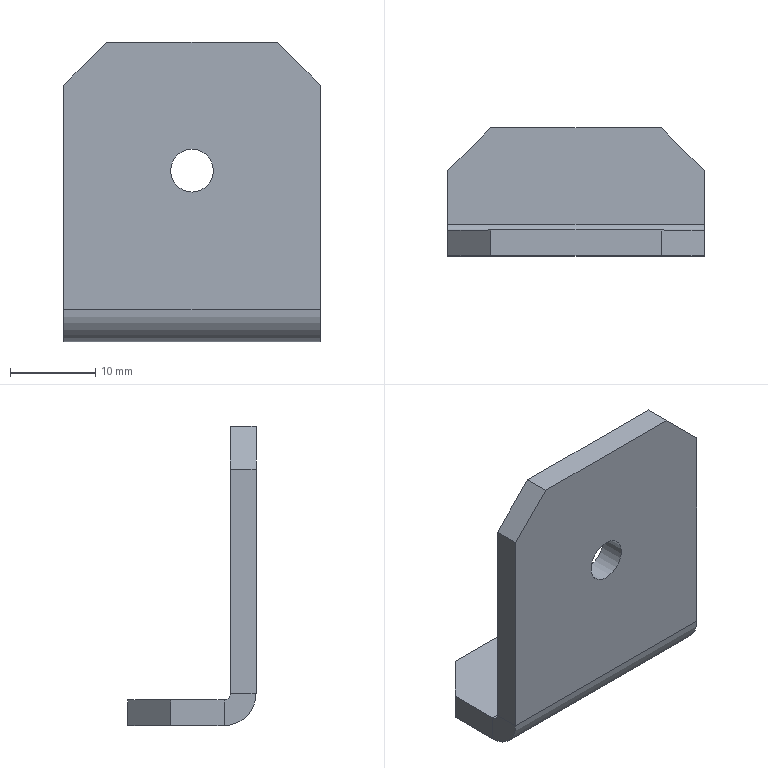Part | NX | 1 solid | 19 faces | box 30 x 15 x 35 mm | volume 3934 mm3 | plane 16 | cylinder 3 | commonest cylinder face diameters 1.5 x1 5 x1 7.5 x1
STEP:
#1=CARTESIAN_POINT('',(15.,0.,3.75));
#2=VERTEX_POINT('',#1);
#3=CARTESIAN_POINT('',(15.,3.,3.75));
#4=VERTEX_POINT('',#3);
#5=CARTESIAN_POINT('',(15.,0.,3.75));
#6=DIRECTION('',(0.,1.,0.));
#7=VECTOR('',#6,1000.);
#8=LINE('',#5,#7);
#9=EDGE_CURVE('',#2,#4,#8,.T.);
#10=ORIENTED_EDGE('',*,*,#9,.F.);
#11=CARTESIAN_POINT('',(15.,3.75,0.));
#12=VERTEX_POINT('',#11);
#13=CARTESIAN_POINT('',(15.,3.75,3.75));
#14=DIRECTION('',(1.,0.,0.));
#15=DIRECTION('',(0.,0.,-1.));
#16=AXIS2_PLACEMENT_3D('',#13,#14,#15);
#17=CIRCLE('',#16,3.75);
#18=EDGE_CURVE('',#12,#2,#17,.F.);
#19=ORIENTED_EDGE('',*,*,#18,.F.);
#20=CARTESIAN_POINT('',(15.,3.75,3.));
#21=VERTEX_POINT('',#20);
#22=CARTESIAN_POINT('',(15.,3.75,3.));
#23=DIRECTION('',(0.,0.,-1.));
#24=VECTOR('',#23,1000.);
#25=LINE('',#22,#24);
#26=EDGE_CURVE('',#21,#12,#25,.T.);
#27=ORIENTED_EDGE('',*,*,#26,.F.);
#28=CARTESIAN_POINT('',(15.,3.75,3.75));
#29=DIRECTION('',(1.,0.,0.));
#30=DIRECTION('',(0.,0.,-1.));
#31=AXIS2_PLACEMENT_3D('',#28,#29,#30);
#32=CIRCLE('',#31,0.75);
#33=EDGE_CURVE('',#21,#4,#32,.F.);
#34=ORIENTED_EDGE('',*,*,#33,.T.);
#35=EDGE_LOOP('',(#10,#19,#27,#34));
#36=FACE_BOUND('',#35,.T.);
#37=CARTESIAN_POINT('',(15.,0.,3.75));
#38=DIRECTION('',(1.,0.,0.));
#39=DIRECTION('',(0.,0.,-1.));
#40=AXIS2_PLACEMENT_3D('',#37,#38,#39);
#41=PLANE('',#40);
#42=ADVANCED_FACE('',(#36),#41,.T.);
#43=CARTESIAN_POINT('',(15.,3.,30.));
#44=VERTEX_POINT('',#43);
#45=CARTESIAN_POINT('',(15.,3.,0.));
#46=DIRECTION('',(0.,0.,1.));
#47=VECTOR('',#46,1000.);
#48=LINE('',#45,#47);
#49=EDGE_CURVE('',#4,#44,#48,.T.);
#50=ORIENTED_EDGE('',*,*,#49,.T.);
#51=CARTESIAN_POINT('',(15.,0.,30.));
#52=VERTEX_POINT('',#51);
#53=CARTESIAN_POINT('',(15.,3.75,30.));
#54=DIRECTION('',(0.,-1.,0.));
#55=VECTOR('',#54,1000.);
#56=LINE('',#53,#55);
#57=EDGE_CURVE('',#44,#52,#56,.T.);
#58=ORIENTED_EDGE('',*,*,#57,.T.);
#59=CARTESIAN_POINT('',(15.,0.,0.));
#60=DIRECTION('',(0.,0.,1.));
#61=VECTOR('',#60,1000.);
#62=LINE('',#59,#61);
#63=EDGE_CURVE('',#2,#52,#62,.T.);
#64=ORIENTED_EDGE('',*,*,#63,.F.);
#65=ORIENTED_EDGE('',*,*,#9,.T.);
#66=EDGE_LOOP('',(#50,#58,#64,#65));
#67=FACE_BOUND('',#66,.T.);
#68=CARTESIAN_POINT('',(15.,3.75,3.));
#69=DIRECTION('',(1.,0.,0.));
#70=DIRECTION('',(0.,0.,-1.));
#71=AXIS2_PLACEMENT_3D('',#68,#69,#70);
#72=PLANE('',#71);
#73=ADVANCED_FACE('',(#67),#72,.T.);
#74=CARTESIAN_POINT('',(-15.,3.75,0.));
#75=VERTEX_POINT('',#74);
#76=CARTESIAN_POINT('',(-15.,3.75,3.));
#77=VERTEX_POINT('',#76);
#78=CARTESIAN_POINT('',(-15.,3.75,0.));
#79=DIRECTION('',(0.,0.,1.));
#80=VECTOR('',#79,1000.);
#81=LINE('',#78,#80);
#82=EDGE_CURVE('',#75,#77,#81,.T.);
#83=ORIENTED_EDGE('',*,*,#82,.F.);
#84=CARTESIAN_POINT('',(-15.,0.,3.75));
#85=VERTEX_POINT('',#84);
#86=CARTESIAN_POINT('',(-15.,3.75,3.75));
#87=DIRECTION('',(1.,0.,0.));
#88=DIRECTION('',(0.,0.,-1.));
#89=AXIS2_PLACEMENT_3D('',#86,#87,#88);
#90=CIRCLE('',#89,3.75);
#91=EDGE_CURVE('',#75,#85,#90,.F.);
#92=ORIENTED_EDGE('',*,*,#91,.T.);
#93=CARTESIAN_POINT('',(-15.,3.,3.75));
#94=VERTEX_POINT('',#93);
#95=CARTESIAN_POINT('',(-15.,3.,3.75));
#96=DIRECTION('',(0.,-1.,0.));
#97=VECTOR('',#96,1000.);
#98=LINE('',#95,#97);
#99=EDGE_CURVE('',#94,#85,#98,.T.);
#100=ORIENTED_EDGE('',*,*,#99,.F.);
#101=CARTESIAN_POINT('',(-15.,3.75,3.75));
#102=DIRECTION('',(1.,0.,0.));
#103=DIRECTION('',(0.,0.,-1.));
#104=AXIS2_PLACEMENT_3D('',#101,#102,#103);
#105=CIRCLE('',#104,0.75);
#106=EDGE_CURVE('',#77,#94,#105,.F.);
#107=ORIENTED_EDGE('',*,*,#106,.F.);
#108=EDGE_LOOP('',(#83,#92,#100,#107));
#109=FACE_BOUND('',#108,.T.);
#110=CARTESIAN_POINT('',(-15.,3.75,0.));
#111=DIRECTION('',(-1.,0.,0.));
#112=DIRECTION('',(0.,0.,1.));
#113=AXIS2_PLACEMENT_3D('',#110,#111,#112);
#114=PLANE('',#113);
#115=ADVANCED_FACE('',(#109),#114,.T.);
#116=CARTESIAN_POINT('',(-15.,10.,3.));
#117=VERTEX_POINT('',#116);
#118=CARTESIAN_POINT('',(-15.,15.,3.));
#119=DIRECTION('',(0.,-1.,0.));
#120=VECTOR('',#119,1000.);
#121=LINE('',#118,#120);
#122=EDGE_CURVE('',#117,#77,#121,.T.);
#123=ORIENTED_EDGE('',*,*,#122,.F.);
#124=CARTESIAN_POINT('',(-15.,10.,0.));
#125=VERTEX_POINT('',#124);
#126=CARTESIAN_POINT('',(-15.,10.,3.75));
#127=DIRECTION('',(0.,0.,-1.));
#128=VECTOR('',#127,1000.);
#129=LINE('',#126,#128);
#130=EDGE_CURVE('',#117,#125,#129,.T.);
#131=ORIENTED_EDGE('',*,*,#130,.T.);
#132=CARTESIAN_POINT('',(-15.,15.,0.));
#133=DIRECTION('',(0.,-1.,0.));
#134=VECTOR('',#133,1000.);
#135=LINE('',#132,#134);
#136=EDGE_CURVE('',#125,#75,#135,.T.);
#137=ORIENTED_EDGE('',*,*,#136,.T.);
#138=ORIENTED_EDGE('',*,*,#82,.T.);
#139=EDGE_LOOP('',(#123,#131,#137,#138));
#140=FACE_BOUND('',#139,.T.);
#141=CARTESIAN_POINT('',(-15.,3.,3.75));
#142=DIRECTION('',(-1.,0.,0.));
#143=DIRECTION('',(0.,0.,1.));
#144=AXIS2_PLACEMENT_3D('',#141,#142,#143);
#145=PLANE('',#144);
#146=ADVANCED_FACE('',(#140),#145,.T.);
#147=CARTESIAN_POINT('',(0.,3.,17.5));
#148=VERTEX_POINT('',#147);
#149=CARTESIAN_POINT('',(0.,3.,20.));
#150=DIRECTION('',(0.,-1.,0.));
#151=DIRECTION('',(0.,0.,-1.));
#152=AXIS2_PLACEMENT_3D('',#149,#150,#151);
#153=CIRCLE('',#152,2.5);
#154=EDGE_CURVE('',#148,#148,#153,.T.);
#155=ORIENTED_EDGE('',*,*,#154,.T.);
#156=EDGE_LOOP('',(#155));
#157=FACE_BOUND('',#156,.T.);
#158=CARTESIAN_POINT('',(10.,3.,35.));
#159=VERTEX_POINT('',#158);
#160=CARTESIAN_POINT('',(-10.,3.,35.));
#161=VERTEX_POINT('',#160);
#162=CARTESIAN_POINT('',(15.,3.,35.));
#163=DIRECTION('',(-1.,0.,0.));
#164=VECTOR('',#163,1000.);
#165=LINE('',#162,#164);
#166=EDGE_CURVE('',#159,#161,#165,.T.);
#167=ORIENTED_EDGE('',*,*,#166,.F.);
#168=CARTESIAN_POINT('',(10.,3.,35.));
#169=DIRECTION('',(-0.7071,0.,0.7071));
#170=VECTOR('',#169,1000.);
#171=LINE('',#168,#170);
#172=EDGE_CURVE('',#159,#44,#171,.F.);
#173=ORIENTED_EDGE('',*,*,#172,.T.);
#174=ORIENTED_EDGE('',*,*,#49,.F.);
#175=CARTESIAN_POINT('',(15.,3.,3.75));
#176=DIRECTION('',(-1.,0.,0.));
#177=VECTOR('',#176,1000.);
#178=LINE('',#175,#177);
#179=EDGE_CURVE('',#4,#94,#178,.T.);
#180=ORIENTED_EDGE('',*,*,#179,.T.);
#181=CARTESIAN_POINT('',(-15.,3.,30.));
#182=VERTEX_POINT('',#181);
#183=CARTESIAN_POINT('',(-15.,3.,0.));
#184=DIRECTION('',(0.,0.,1.));
#185=VECTOR('',#184,1000.);
#186=LINE('',#183,#185);
#187=EDGE_CURVE('',#94,#182,#186,.T.);
#188=ORIENTED_EDGE('',*,*,#187,.T.);
#189=CARTESIAN_POINT('',(-15.,3.,30.));
#190=DIRECTION('',(0.7071,0.,0.7071));
#191=VECTOR('',#190,1000.);
#192=LINE('',#189,#191);
#193=EDGE_CURVE('',#182,#161,#192,.T.);
#194=ORIENTED_EDGE('',*,*,#193,.T.);
#195=EDGE_LOOP('',(#167,#173,#174,#180,#188,#194));
#196=FACE_BOUND('',#195,.T.);
#197=CARTESIAN_POINT('',(15.,3.,0.));
#198=DIRECTION('',(0.,-1.,0.));
#199=DIRECTION('',(0.,0.,-1.));
#200=AXIS2_PLACEMENT_3D('',#197,#198,#199);
#201=PLANE('',#200);
#202=ADVANCED_FACE('',(#157,#196),#201,.F.);
#203=CARTESIAN_POINT('',(10.,0.,35.));
#204=VERTEX_POINT('',#203);
#205=CARTESIAN_POINT('',(-10.,0.,35.));
#206=VERTEX_POINT('',#205);
#207=CARTESIAN_POINT('',(15.,0.,35.));
#208=DIRECTION('',(-1.,0.,0.));
#209=VECTOR('',#208,1000.);
#210=LINE('',#207,#209);
#211=EDGE_CURVE('',#204,#206,#210,.T.);
#212=ORIENTED_EDGE('',*,*,#211,.F.);
#213=CARTESIAN_POINT('',(10.,0.,35.));
#214=DIRECTION('',(0.,1.,0.));
#215=VECTOR('',#214,1000.);
#216=LINE('',#213,#215);
#217=EDGE_CURVE('',#204,#159,#216,.T.);
#218=ORIENTED_EDGE('',*,*,#217,.T.);
#219=ORIENTED_EDGE('',*,*,#166,.T.);
#220=CARTESIAN_POINT('',(-10.,0.,35.));
#221=DIRECTION('',(0.,-1.,0.));
#222=VECTOR('',#221,1000.);
#223=LINE('',#220,#222);
#224=EDGE_CURVE('',#161,#206,#223,.T.);
#225=ORIENTED_EDGE('',*,*,#224,.T.);
#226=EDGE_LOOP('',(#212,#218,#219,#225));
#227=FACE_BOUND('',#226,.T.);
#228=CARTESIAN_POINT('',(15.,0.,35.));
#229=DIRECTION('',(0.,0.,1.));
#230=DIRECTION('',(1.,0.,0.));
#231=AXIS2_PLACEMENT_3D('',#228,#229,#230);
#232=PLANE('',#231);
#233=ADVANCED_FACE('',(#227),#232,.T.);
#234=CARTESIAN_POINT('',(0.,0.,17.5));
#235=VERTEX_POINT('',#234);
#236=CARTESIAN_POINT('',(0.,0.,20.));
#237=DIRECTION('',(0.,-1.,0.));
#238=DIRECTION('',(0.,0.,-1.));
#239=AXIS2_PLACEMENT_3D('',#236,#237,#238);
#240=CIRCLE('',#239,2.5);
#241=EDGE_CURVE('',#235,#235,#240,.T.);
#242=ORIENTED_EDGE('',*,*,#241,.F.);
#243=EDGE_LOOP('',(#242));
#244=FACE_BOUND('',#243,.T.);
#245=ORIENTED_EDGE('',*,*,#63,.T.);
#246=CARTESIAN_POINT('',(30.,0.,15.));
#247=DIRECTION('',(0.7071,0.,-0.7071));
#248=VECTOR('',#247,1000.);
#249=LINE('',#246,#248);
#250=EDGE_CURVE('',#52,#204,#249,.F.);
#251=ORIENTED_EDGE('',*,*,#250,.T.);
#252=ORIENTED_EDGE('',*,*,#211,.T.);
#253=CARTESIAN_POINT('',(-15.,0.,30.));
#254=VERTEX_POINT('',#253);
#255=CARTESIAN_POINT('',(-15.,0.,30.));
#256=DIRECTION('',(-0.7071,0.,-0.7071));
#257=VECTOR('',#256,1000.);
#258=LINE('',#255,#257);
#259=EDGE_CURVE('',#206,#254,#258,.T.);
#260=ORIENTED_EDGE('',*,*,#259,.T.);
#261=CARTESIAN_POINT('',(-15.,0.,0.));
#262=DIRECTION('',(0.,0.,1.));
#263=VECTOR('',#262,1000.);
#264=LINE('',#261,#263);
#265=EDGE_CURVE('',#85,#254,#264,.T.);
#266=ORIENTED_EDGE('',*,*,#265,.F.);
#267=CARTESIAN_POINT('',(15.,0.,3.75));
#268=DIRECTION('',(-1.,0.,0.));
#269=VECTOR('',#268,1000.);
#270=LINE('',#267,#269);
#271=EDGE_CURVE('',#2,#85,#270,.T.);
#272=ORIENTED_EDGE('',*,*,#271,.F.);
#273=EDGE_LOOP('',(#245,#251,#252,#260,#266,#272));
#274=FACE_BOUND('',#273,.T.);
#275=CARTESIAN_POINT('',(15.,0.,0.));
#276=DIRECTION('',(0.,-1.,0.));
#277=DIRECTION('',(0.,0.,-1.));
#278=AXIS2_PLACEMENT_3D('',#275,#276,#277);
#279=PLANE('',#278);
#280=ADVANCED_FACE('',(#244,#274),#279,.T.);
#281=ORIENTED_EDGE('',*,*,#91,.F.);
#282=CARTESIAN_POINT('',(15.,3.75,0.));
#283=DIRECTION('',(-1.,0.,0.));
#284=VECTOR('',#283,1000.);
#285=LINE('',#282,#284);
#286=EDGE_CURVE('',#12,#75,#285,.T.);
#287=ORIENTED_EDGE('',*,*,#286,.F.);
#288=ORIENTED_EDGE('',*,*,#18,.T.);
#289=ORIENTED_EDGE('',*,*,#271,.T.);
#290=EDGE_LOOP('',(#281,#287,#288,#289));
#291=FACE_BOUND('',#290,.T.);
#292=CARTESIAN_POINT('',(15.,3.75,3.75));
#293=DIRECTION('',(-1.,0.,0.));
#294=DIRECTION('',(0.,0.,1.));
#295=AXIS2_PLACEMENT_3D('',#292,#293,#294);
#296=CYLINDRICAL_SURFACE('',#295,3.75);
#297=ADVANCED_FACE('',(#291),#296,.T.);
#298=CARTESIAN_POINT('',(10.,15.,0.));
#299=VERTEX_POINT('',#298);
#300=CARTESIAN_POINT('',(-10.,15.,0.));
#301=VERTEX_POINT('',#300);
#302=CARTESIAN_POINT('',(15.,15.,0.));
#303=DIRECTION('',(-1.,0.,0.));
#304=VECTOR('',#303,1000.);
#305=LINE('',#302,#304);
#306=EDGE_CURVE('',#299,#301,#305,.T.);
#307=ORIENTED_EDGE('',*,*,#306,.F.);
#308=CARTESIAN_POINT('',(15.,10.,0.));
#309=VERTEX_POINT('',#308);
#310=CARTESIAN_POINT('',(12.5,12.5,0.));
#311=DIRECTION('',(-0.7071,0.7071,0.));
#312=VECTOR('',#311,1000.);
#313=LINE('',#310,#312);
#314=EDGE_CURVE('',#299,#309,#313,.F.);
#315=ORIENTED_EDGE('',*,*,#314,.T.);
#316=CARTESIAN_POINT('',(15.,15.,0.));
#317=DIRECTION('',(0.,-1.,0.));
#318=VECTOR('',#317,1000.);
#319=LINE('',#316,#318);
#320=EDGE_CURVE('',#309,#12,#319,.T.);
#321=ORIENTED_EDGE('',*,*,#320,.T.);
#322=ORIENTED_EDGE('',*,*,#286,.T.);
#323=ORIENTED_EDGE('',*,*,#136,.F.);
#324=CARTESIAN_POINT('',(2.5,27.5,0.));
#325=DIRECTION('',(-0.7071,-0.7071,0.));
#326=VECTOR('',#325,1000.);
#327=LINE('',#324,#326);
#328=EDGE_CURVE('',#125,#301,#327,.F.);
#329=ORIENTED_EDGE('',*,*,#328,.T.);
#330=EDGE_LOOP('',(#307,#315,#321,#322,#323,#329));
#331=FACE_BOUND('',#330,.T.);
#332=CARTESIAN_POINT('',(15.,15.,0.));
#333=DIRECTION('',(0.,0.,-1.));
#334=DIRECTION('',(0.,1.,0.));
#335=AXIS2_PLACEMENT_3D('',#332,#333,#334);
#336=PLANE('',#335);
#337=ADVANCED_FACE('',(#331),#336,.T.);
#338=CARTESIAN_POINT('',(10.,15.,3.));
#339=VERTEX_POINT('',#338);
#340=CARTESIAN_POINT('',(-10.,15.,3.));
#341=VERTEX_POINT('',#340);
#342=CARTESIAN_POINT('',(15.,15.,3.));
#343=DIRECTION('',(-1.,0.,0.));
#344=VECTOR('',#343,1000.);
#345=LINE('',#342,#344);
#346=EDGE_CURVE('',#339,#341,#345,.T.);
#347=ORIENTED_EDGE('',*,*,#346,.F.);
#348=CARTESIAN_POINT('',(10.,15.,3.));
#349=DIRECTION('',(0.,0.,-1.));
#350=VECTOR('',#349,1000.);
#351=LINE('',#348,#350);
#352=EDGE_CURVE('',#339,#299,#351,.T.);
#353=ORIENTED_EDGE('',*,*,#352,.T.);
#354=ORIENTED_EDGE('',*,*,#306,.T.);
#355=CARTESIAN_POINT('',(-10.,15.,3.));
#356=DIRECTION('',(0.,0.,1.));
#357=VECTOR('',#356,1000.);
#358=LINE('',#355,#357);
#359=EDGE_CURVE('',#301,#341,#358,.T.);
#360=ORIENTED_EDGE('',*,*,#359,.T.);
#361=EDGE_LOOP('',(#347,#353,#354,#360));
#362=FACE_BOUND('',#361,.T.);
#363=CARTESIAN_POINT('',(15.,15.,3.));
#364=DIRECTION('',(0.,1.,0.));
#365=DIRECTION('',(0.,0.,1.));
#366=AXIS2_PLACEMENT_3D('',#363,#364,#365);
#367=PLANE('',#366);
#368=ADVANCED_FACE('',(#362),#367,.T.);
#369=CARTESIAN_POINT('',(15.,10.,3.));
#370=VERTEX_POINT('',#369);
#371=CARTESIAN_POINT('',(15.,15.,3.));
#372=DIRECTION('',(0.,-1.,0.));
#373=VECTOR('',#372,1000.);
#374=LINE('',#371,#373);
#375=EDGE_CURVE('',#370,#21,#374,.T.);
#376=ORIENTED_EDGE('',*,*,#375,.F.);
#377=CARTESIAN_POINT('',(10.,15.,3.));
#378=DIRECTION('',(0.7071,-0.7071,0.));
#379=VECTOR('',#378,1000.);
#380=LINE('',#377,#379);
#381=EDGE_CURVE('',#370,#339,#380,.F.);
#382=ORIENTED_EDGE('',*,*,#381,.T.);
#383=ORIENTED_EDGE('',*,*,#346,.T.);
#384=CARTESIAN_POINT('',(-15.,10.,3.));
#385=DIRECTION('',(0.7071,0.7071,0.));
#386=VECTOR('',#385,1000.);
#387=LINE('',#384,#386);
#388=EDGE_CURVE('',#341,#117,#387,.F.);
#389=ORIENTED_EDGE('',*,*,#388,.T.);
#390=ORIENTED_EDGE('',*,*,#122,.T.);
#391=CARTESIAN_POINT('',(15.,3.75,3.));
#392=DIRECTION('',(-1.,0.,0.));
#393=VECTOR('',#392,1000.);
#394=LINE('',#391,#393);
#395=EDGE_CURVE('',#21,#77,#394,.T.);
#396=ORIENTED_EDGE('',*,*,#395,.F.);
#397=EDGE_LOOP('',(#376,#382,#383,#389,#390,#396));
#398=FACE_BOUND('',#397,.T.);
#399=CARTESIAN_POINT('',(15.,15.,3.));
#400=DIRECTION('',(0.,0.,-1.));
#401=DIRECTION('',(0.,1.,0.));
#402=AXIS2_PLACEMENT_3D('',#399,#400,#401);
#403=PLANE('',#402);
#404=ADVANCED_FACE('',(#398),#403,.F.);
#405=ORIENTED_EDGE('',*,*,#106,.T.);
#406=ORIENTED_EDGE('',*,*,#179,.F.);
#407=ORIENTED_EDGE('',*,*,#33,.F.);
#408=ORIENTED_EDGE('',*,*,#395,.T.);
#409=EDGE_LOOP('',(#405,#406,#407,#408));
#410=FACE_BOUND('',#409,.T.);
#411=CARTESIAN_POINT('',(15.,3.75,3.75));
#412=DIRECTION('',(-1.,0.,0.));
#413=DIRECTION('',(0.,0.,1.));
#414=AXIS2_PLACEMENT_3D('',#411,#412,#413);
#415=CYLINDRICAL_SURFACE('',#414,0.75);
#416=ADVANCED_FACE('',(#410),#415,.F.);
#417=ORIENTED_EDGE('',*,*,#320,.F.);
#418=CARTESIAN_POINT('',(15.,10.,3.75));
#419=DIRECTION('',(0.,0.,1.));
#420=VECTOR('',#419,1000.);
#421=LINE('',#418,#420);
#422=EDGE_CURVE('',#309,#370,#421,.T.);
#423=ORIENTED_EDGE('',*,*,#422,.T.);
#424=ORIENTED_EDGE('',*,*,#375,.T.);
#425=ORIENTED_EDGE('',*,*,#26,.T.);
#426=EDGE_LOOP('',(#417,#423,#424,#425));
#427=FACE_BOUND('',#426,.T.);
#428=CARTESIAN_POINT('',(15.,3.75,3.75));
#429=DIRECTION('',(1.,0.,0.));
#430=DIRECTION('',(0.,0.,-1.));
#431=AXIS2_PLACEMENT_3D('',#428,#429,#430);
#432=PLANE('',#431);
#433=ADVANCED_FACE('',(#427),#432,.T.);
#434=ORIENTED_EDGE('',*,*,#265,.T.);
#435=CARTESIAN_POINT('',(-15.,3.,30.));
#436=DIRECTION('',(0.,1.,0.));
#437=VECTOR('',#436,1000.);
#438=LINE('',#435,#437);
#439=EDGE_CURVE('',#254,#182,#438,.T.);
#440=ORIENTED_EDGE('',*,*,#439,.T.);
#441=ORIENTED_EDGE('',*,*,#187,.F.);
#442=ORIENTED_EDGE('',*,*,#99,.T.);
#443=EDGE_LOOP('',(#434,#440,#441,#442));
#444=FACE_BOUND('',#443,.T.);
#445=CARTESIAN_POINT('',(-15.,3.75,3.75));
#446=DIRECTION('',(1.,0.,0.));
#447=DIRECTION('',(0.,0.,-1.));
#448=AXIS2_PLACEMENT_3D('',#445,#446,#447);
#449=PLANE('',#448);
#450=ADVANCED_FACE('',(#444),#449,.F.);
#451=ORIENTED_EDGE('',*,*,#241,.T.);
#452=EDGE_LOOP('',(#451));
#453=FACE_BOUND('',#452,.T.);
#454=ORIENTED_EDGE('',*,*,#154,.F.);
#455=EDGE_LOOP('',(#454));
#456=FACE_BOUND('',#455,.T.);
#457=CARTESIAN_POINT('',(0.,0.,20.));
#458=DIRECTION('',(0.,-1.,0.));
#459=DIRECTION('',(0.,0.,-1.));
#460=AXIS2_PLACEMENT_3D('',#457,#458,#459);
#461=CYLINDRICAL_SURFACE('',#460,2.5);
#462=ADVANCED_FACE('',(#453,#456),#461,.F.);
#463=ORIENTED_EDGE('',*,*,#381,.F.);
#464=ORIENTED_EDGE('',*,*,#422,.F.);
#465=ORIENTED_EDGE('',*,*,#314,.F.);
#466=ORIENTED_EDGE('',*,*,#352,.F.);
#467=EDGE_LOOP('',(#463,#464,#465,#466));
#468=FACE_BOUND('',#467,.T.);
#469=CARTESIAN_POINT('',(10.,15.,3.));
#470=DIRECTION('',(-0.7071,-0.7071,0.));
#471=DIRECTION('',(0.,0.,-1.));
#472=AXIS2_PLACEMENT_3D('',#469,#470,#471);
#473=PLANE('',#472);
#474=ADVANCED_FACE('',(#468),#473,.F.);
#475=ORIENTED_EDGE('',*,*,#388,.F.);
#476=ORIENTED_EDGE('',*,*,#359,.F.);
#477=ORIENTED_EDGE('',*,*,#328,.F.);
#478=ORIENTED_EDGE('',*,*,#130,.F.);
#479=EDGE_LOOP('',(#475,#476,#477,#478));
#480=FACE_BOUND('',#479,.T.);
#481=CARTESIAN_POINT('',(-15.,10.,3.75));
#482=DIRECTION('',(0.7071,-0.7071,0.));
#483=DIRECTION('',(0.,0.,-1.));
#484=AXIS2_PLACEMENT_3D('',#481,#482,#483);
#485=PLANE('',#484);
#486=ADVANCED_FACE('',(#480),#485,.F.);
#487=ORIENTED_EDGE('',*,*,#250,.F.);
#488=ORIENTED_EDGE('',*,*,#57,.F.);
#489=ORIENTED_EDGE('',*,*,#172,.F.);
#490=ORIENTED_EDGE('',*,*,#217,.F.);
#491=EDGE_LOOP('',(#487,#488,#489,#490));
#492=FACE_BOUND('',#491,.T.);
#493=CARTESIAN_POINT('',(10.,0.,35.));
#494=DIRECTION('',(-0.7071,0.,-0.7071));
#495=DIRECTION('',(0.,1.,0.));
#496=AXIS2_PLACEMENT_3D('',#493,#494,#495);
#497=PLANE('',#496);
#498=ADVANCED_FACE('',(#492),#497,.F.);
#499=ORIENTED_EDGE('',*,*,#259,.F.);
#500=ORIENTED_EDGE('',*,*,#224,.F.);
#501=ORIENTED_EDGE('',*,*,#193,.F.);
#502=ORIENTED_EDGE('',*,*,#439,.F.);
#503=EDGE_LOOP('',(#499,#500,#501,#502));
#504=FACE_BOUND('',#503,.T.);
#505=CARTESIAN_POINT('',(-15.,3.75,30.));
#506=DIRECTION('',(-0.7071,0.,0.7071));
#507=DIRECTION('',(0.,-1.,0.));
#508=AXIS2_PLACEMENT_3D('',#505,#506,#507);
#509=PLANE('',#508);
#510=ADVANCED_FACE('',(#504),#509,.T.);
#511=CLOSED_SHELL('',(#42,#73,#115,#146,#202,#233,#280,#297,#337,#368,#404,#416,#433,#450,#462,#474,#486,#498,#510));
#512=MANIFOLD_SOLID_BREP('',#511);
#513=(LENGTH_UNIT()NAMED_UNIT(*)SI_UNIT(.MILLI.,.METRE.));
#514=UNCERTAINTY_MEASURE_WITH_UNIT(LENGTH_MEASURE(0.00001),#513,'','');
#515=(NAMED_UNIT(*)PLANE_ANGLE_UNIT()SI_UNIT($,.RADIAN.));
#516=(NAMED_UNIT(*)SI_UNIT($,.STERADIAN.)SOLID_ANGLE_UNIT());
#517=(GEOMETRIC_REPRESENTATION_CONTEXT(3)GLOBAL_UNCERTAINTY_ASSIGNED_CONTEXT((#514))GLOBAL_UNIT_ASSIGNED_CONTEXT((#513,#515,#516))REPRESENTATION_CONTEXT('',''));
#518=ADVANCED_BREP_SHAPE_REPRESENTATION('',(#512),#517);